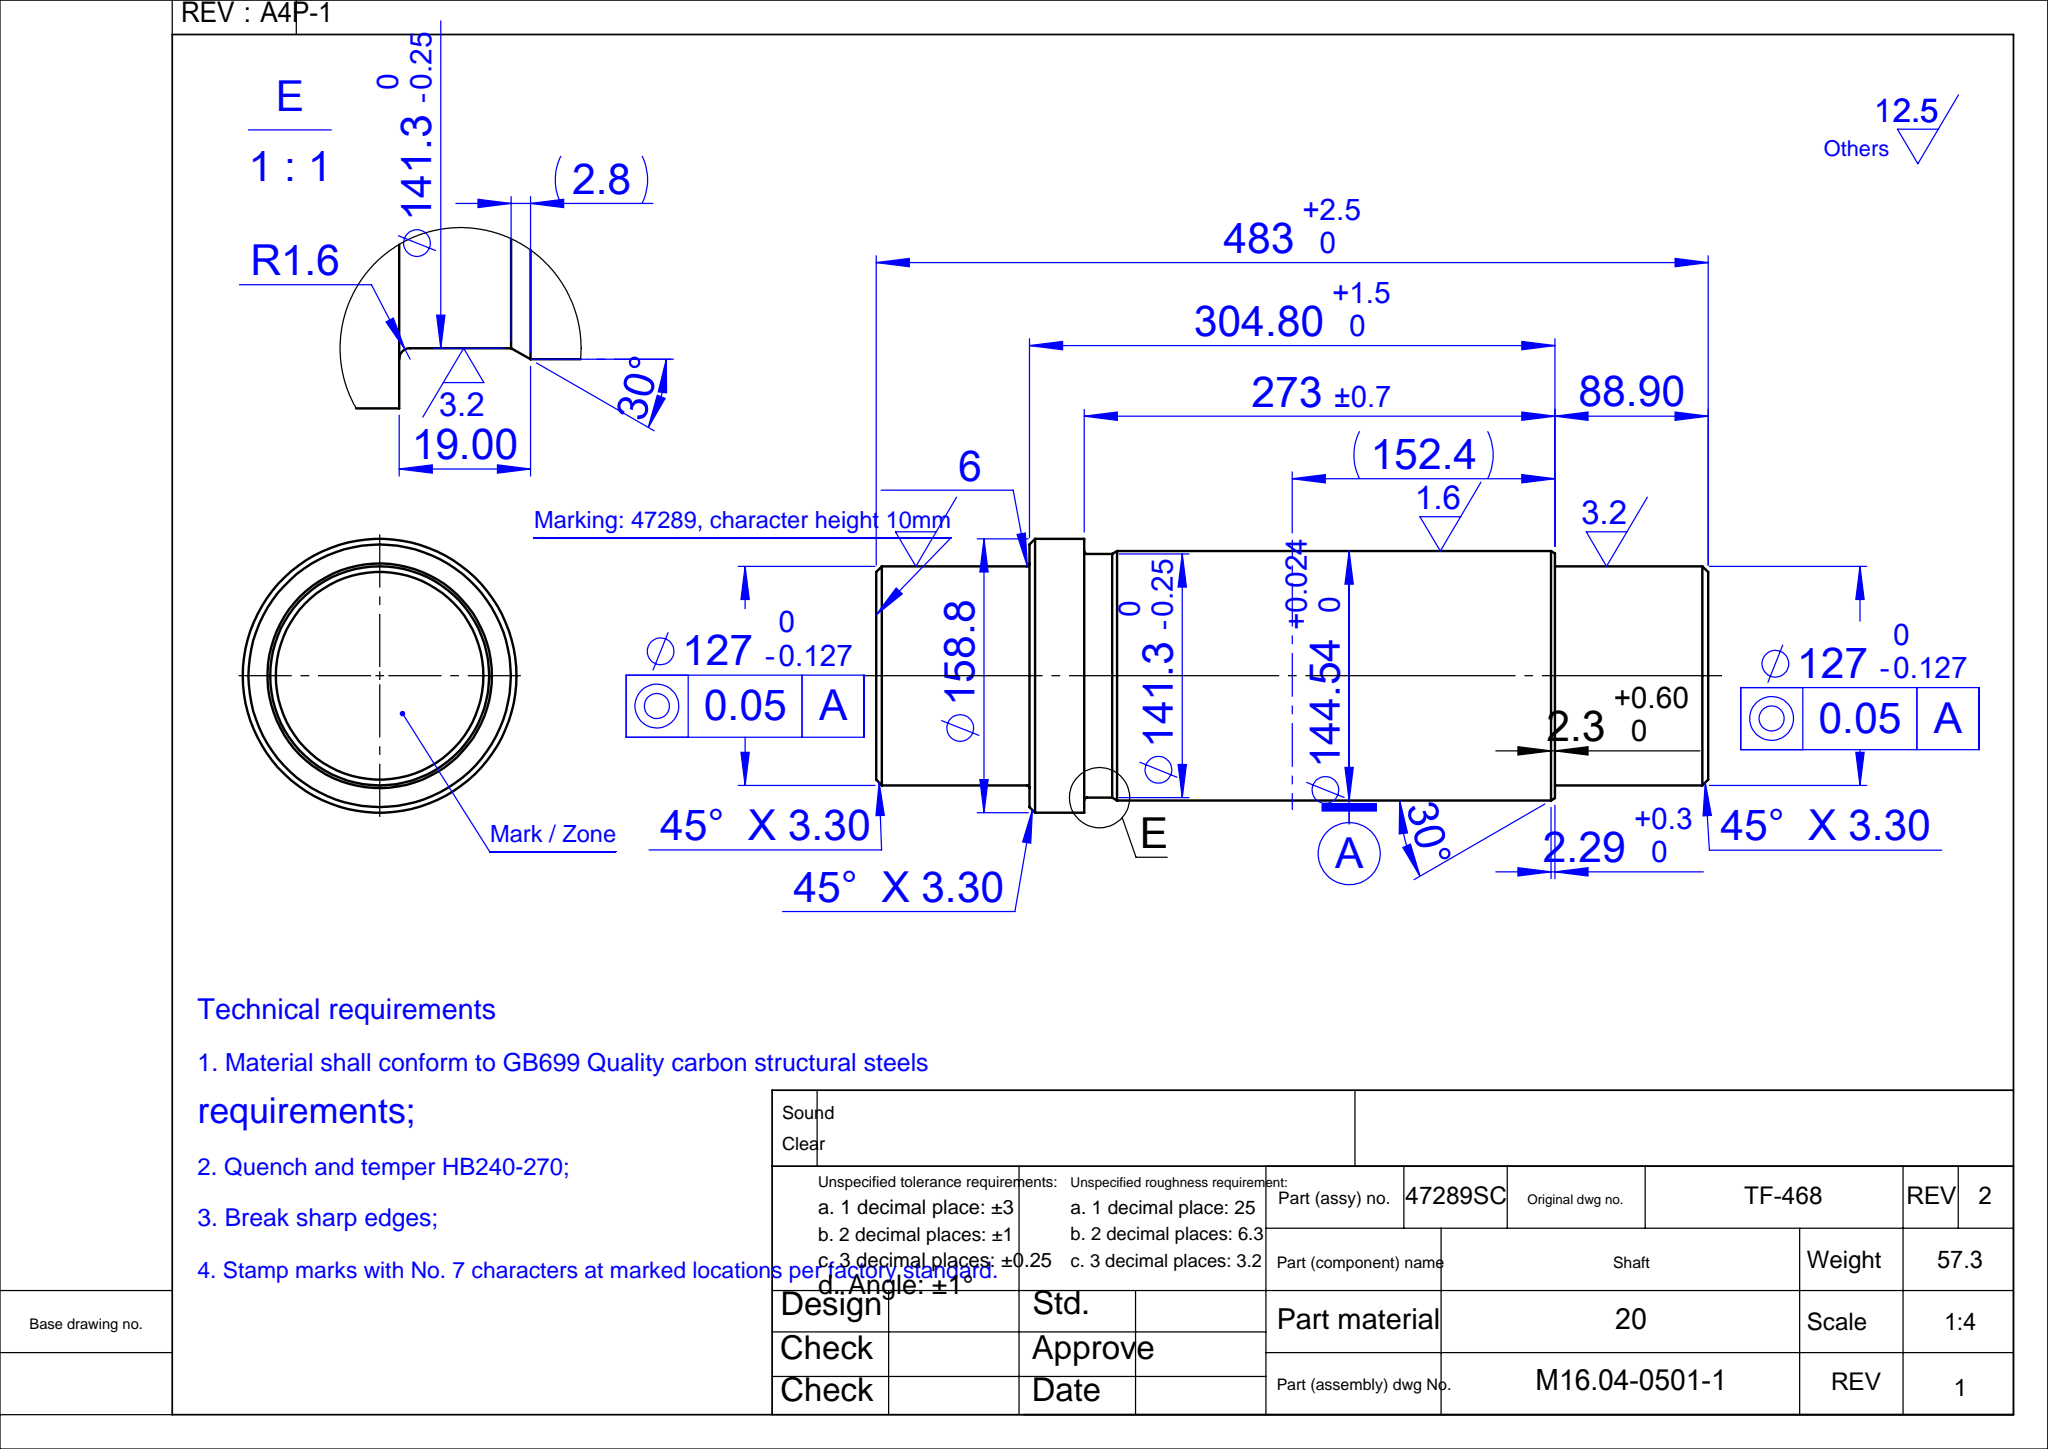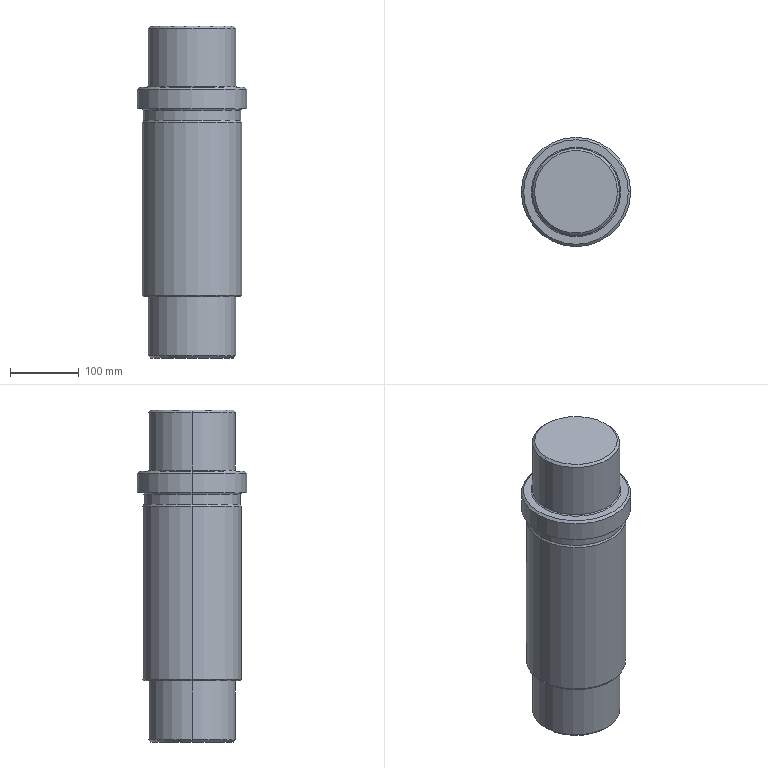Part | SolidWorks | features Revolution 1 | 1 solid | 29 faces | box 158.75 x 158.75 x 482.6 mm | volume 7340968 mm3 | cylinder 10 | cone 10 | plane 5 | torus 4 | commonest cylinder face diameters 127 x4 141.3 x2 144.539 x2 158.75 x2
STEP:
#1=CARTESIAN_POINT('',(-72.238,0.,120.65));
#2=VERTEX_POINT('',#1);
#3=CARTESIAN_POINT('',(72.238,0.,120.65));
#4=VERTEX_POINT('',#3);
#5=CARTESIAN_POINT('',(0.,0.,120.65));
#6=DIRECTION('',(0.,0.,1.));
#7=DIRECTION('',(1.,0.,0.));
#8=AXIS2_PLACEMENT_3D('',#5,#6,#7);
#9=CIRCLE('',#8,72.238);
#10=EDGE_CURVE('',#2,#4,#9,.T.);
#11=ORIENTED_EDGE('',*,*,#10,.F.);
#12=CARTESIAN_POINT('',(-70.65,0.,119.063));
#13=VERTEX_POINT('',#12);
#14=CARTESIAN_POINT('',(-72.238,0.,119.062));
#15=DIRECTION('',(0.,1.,0.));
#16=DIRECTION('',(-1.,0.,0.));
#17=AXIS2_PLACEMENT_3D('',#14,#15,#16);
#18=CIRCLE('',#17,1.588);
#19=EDGE_CURVE('',#2,#13,#18,.T.);
#20=ORIENTED_EDGE('',*,*,#19,.T.);
#21=CARTESIAN_POINT('',(70.65,0.,119.063));
#22=VERTEX_POINT('',#21);
#23=CARTESIAN_POINT('',(0.,0.,119.063));
#24=DIRECTION('',(0.,0.,1.));
#25=DIRECTION('',(1.,0.,0.));
#26=AXIS2_PLACEMENT_3D('',#23,#24,#25);
#27=CIRCLE('',#26,70.65);
#28=EDGE_CURVE('',#13,#22,#27,.T.);
#29=ORIENTED_EDGE('',*,*,#28,.T.);
#30=CARTESIAN_POINT('',(72.238,0.,119.062));
#31=DIRECTION('',(0.,-1.,0.));
#32=DIRECTION('',(0.,0.,-1.));
#33=AXIS2_PLACEMENT_3D('',#30,#31,#32);
#34=CIRCLE('',#33,1.588);
#35=EDGE_CURVE('',#4,#22,#34,.T.);
#36=ORIENTED_EDGE('',*,*,#35,.F.);
#37=EDGE_LOOP('',(#11,#20,#29,#36));
#38=FACE_OUTER_BOUND('',#37,.T.);
#39=CARTESIAN_POINT('',(0.,0.,119.062));
#40=DIRECTION('',(0.,0.,1.));
#41=DIRECTION('',(1.,0.,0.));
#42=AXIS2_PLACEMENT_3D('',#39,#40,#41);
#43=TOROIDAL_SURFACE('',#42,72.238,1.588);
#44=ADVANCED_FACE('',(#38),#43,.F.);
#45=CARTESIAN_POINT('',(70.65,0.,104.405));
#46=VERTEX_POINT('',#45);
#47=CARTESIAN_POINT('',(-70.65,0.,104.405));
#48=VERTEX_POINT('',#47);
#49=CARTESIAN_POINT('',(0.,0.,104.405));
#50=DIRECTION('',(0.,0.,1.));
#51=DIRECTION('',(1.,0.,0.));
#52=AXIS2_PLACEMENT_3D('',#49,#50,#51);
#53=CIRCLE('',#52,70.65);
#54=EDGE_CURVE('',#46,#48,#53,.T.);
#55=ORIENTED_EDGE('',*,*,#54,.T.);
#56=CARTESIAN_POINT('',(-70.65,0.,264.579));
#57=DIRECTION('',(0.,0.,1.));
#58=VECTOR('',#57,1000.);
#59=LINE('',#56,#58);
#60=EDGE_CURVE('',#48,#13,#59,.T.);
#61=ORIENTED_EDGE('',*,*,#60,.T.);
#62=CARTESIAN_POINT('',(0.,0.,119.063));
#63=DIRECTION('',(0.,0.,1.));
#64=DIRECTION('',(1.,0.,0.));
#65=AXIS2_PLACEMENT_3D('',#62,#63,#64);
#66=CIRCLE('',#65,70.65);
#67=EDGE_CURVE('',#22,#13,#66,.T.);
#68=ORIENTED_EDGE('',*,*,#67,.F.);
#69=CARTESIAN_POINT('',(70.65,0.,264.579));
#70=DIRECTION('',(0.,0.,1.));
#71=VECTOR('',#70,1000.);
#72=LINE('',#69,#71);
#73=EDGE_CURVE('',#46,#22,#72,.T.);
#74=ORIENTED_EDGE('',*,*,#73,.F.);
#75=EDGE_LOOP('',(#55,#61,#68,#74));
#76=FACE_OUTER_BOUND('',#75,.T.);
#77=CARTESIAN_POINT('',(0.,0.,264.579));
#78=DIRECTION('',(0.,0.,1.));
#79=DIRECTION('',(1.,0.,0.));
#80=AXIS2_PLACEMENT_3D('',#77,#78,#79);
#81=CYLINDRICAL_SURFACE('',#80,70.65);
#82=ADVANCED_FACE('',(#76),#81,.T.);
#83=ORIENTED_EDGE('',*,*,#54,.F.);
#84=CARTESIAN_POINT('',(72.269,0.,101.6));
#85=VERTEX_POINT('',#84);
#86=CARTESIAN_POINT('',(72.269,0.,101.6));
#87=DIRECTION('',(0.5,0.,-0.866));
#88=VECTOR('',#87,1000.);
#89=LINE('',#86,#88);
#90=EDGE_CURVE('',#46,#85,#89,.T.);
#91=ORIENTED_EDGE('',*,*,#90,.T.);
#92=CARTESIAN_POINT('',(-72.269,0.,101.6));
#93=VERTEX_POINT('',#92);
#94=CARTESIAN_POINT('',(0.,0.,101.6));
#95=DIRECTION('',(0.,0.,1.));
#96=DIRECTION('',(1.,0.,0.));
#97=AXIS2_PLACEMENT_3D('',#94,#95,#96);
#98=CIRCLE('',#97,72.269);
#99=EDGE_CURVE('',#85,#93,#98,.T.);
#100=ORIENTED_EDGE('',*,*,#99,.T.);
#101=CARTESIAN_POINT('',(-72.269,0.,101.6));
#102=DIRECTION('',(-0.5,0.,-0.866));
#103=VECTOR('',#102,1000.);
#104=LINE('',#101,#103);
#105=EDGE_CURVE('',#48,#93,#104,.T.);
#106=ORIENTED_EDGE('',*,*,#105,.F.);
#107=EDGE_LOOP('',(#83,#91,#100,#106));
#108=FACE_OUTER_BOUND('',#107,.T.);
#109=CARTESIAN_POINT('',(0.,0.,101.6));
#110=DIRECTION('',(0.,0.,-1.));
#111=DIRECTION('',(-1.,0.,0.));
#112=AXIS2_PLACEMENT_3D('',#109,#110,#111);
#113=CONICAL_SURFACE('',#112,72.269,0.5236);
#114=ADVANCED_FACE('',(#108),#113,.T.);
#115=CARTESIAN_POINT('',(72.269,0.,-150.114));
#116=VERTEX_POINT('',#115);
#117=CARTESIAN_POINT('',(-72.269,0.,-150.114));
#118=VERTEX_POINT('',#117);
#119=CARTESIAN_POINT('',(0.,0.,-150.114));
#120=DIRECTION('',(0.,0.,1.));
#121=DIRECTION('',(1.,0.,0.));
#122=AXIS2_PLACEMENT_3D('',#119,#120,#121);
#123=CIRCLE('',#122,72.269);
#124=EDGE_CURVE('',#116,#118,#123,.T.);
#125=ORIENTED_EDGE('',*,*,#124,.T.);
#126=CARTESIAN_POINT('',(-72.269,0.,264.579));
#127=DIRECTION('',(0.,0.,1.));
#128=VECTOR('',#127,1000.);
#129=LINE('',#126,#128);
#130=EDGE_CURVE('',#118,#93,#129,.T.);
#131=ORIENTED_EDGE('',*,*,#130,.T.);
#132=ORIENTED_EDGE('',*,*,#99,.F.);
#133=CARTESIAN_POINT('',(72.269,0.,264.579));
#134=DIRECTION('',(0.,0.,1.));
#135=VECTOR('',#134,1000.);
#136=LINE('',#133,#135);
#137=EDGE_CURVE('',#116,#85,#136,.T.);
#138=ORIENTED_EDGE('',*,*,#137,.F.);
#139=EDGE_LOOP('',(#125,#131,#132,#138));
#140=FACE_OUTER_BOUND('',#139,.T.);
#141=CARTESIAN_POINT('',(0.,0.,264.579));
#142=DIRECTION('',(0.,0.,1.));
#143=DIRECTION('',(1.,0.,0.));
#144=AXIS2_PLACEMENT_3D('',#141,#142,#143);
#145=CYLINDRICAL_SURFACE('',#144,72.269);
#146=ADVANCED_FACE('',(#140),#145,.T.);
#147=CARTESIAN_POINT('',(70.95,0.,-152.4));
#148=VERTEX_POINT('',#147);
#149=CARTESIAN_POINT('',(-70.95,0.,-152.4));
#150=VERTEX_POINT('',#149);
#151=CARTESIAN_POINT('',(0.,0.,-152.4));
#152=DIRECTION('',(0.,0.,1.));
#153=DIRECTION('',(1.,0.,0.));
#154=AXIS2_PLACEMENT_3D('',#151,#152,#153);
#155=CIRCLE('',#154,70.95);
#156=EDGE_CURVE('',#148,#150,#155,.T.);
#157=ORIENTED_EDGE('',*,*,#156,.T.);
#158=CARTESIAN_POINT('',(-70.95,0.,-152.4));
#159=DIRECTION('',(-0.5,0.,0.866));
#160=VECTOR('',#159,1000.);
#161=LINE('',#158,#160);
#162=EDGE_CURVE('',#150,#118,#161,.T.);
#163=ORIENTED_EDGE('',*,*,#162,.T.);
#164=ORIENTED_EDGE('',*,*,#124,.F.);
#165=CARTESIAN_POINT('',(70.95,0.,-152.4));
#166=DIRECTION('',(0.5,0.,0.866));
#167=VECTOR('',#166,1000.);
#168=LINE('',#165,#167);
#169=EDGE_CURVE('',#148,#116,#168,.T.);
#170=ORIENTED_EDGE('',*,*,#169,.F.);
#171=EDGE_LOOP('',(#157,#163,#164,#170));
#172=FACE_OUTER_BOUND('',#171,.T.);
#173=CARTESIAN_POINT('',(0.,0.,-152.4));
#174=DIRECTION('',(0.,0.,1.));
#175=DIRECTION('',(1.,0.,0.));
#176=AXIS2_PLACEMENT_3D('',#173,#174,#175);
#177=CONICAL_SURFACE('',#176,70.95,0.5236);
#178=ADVANCED_FACE('',(#172),#177,.T.);
#179=CARTESIAN_POINT('',(63.5,0.,-237.998));
#180=VERTEX_POINT('',#179);
#181=CARTESIAN_POINT('',(-63.5,0.,-237.998));
#182=VERTEX_POINT('',#181);
#183=CARTESIAN_POINT('',(0.,0.,-237.998));
#184=DIRECTION('',(0.,0.,1.));
#185=DIRECTION('',(1.,0.,0.));
#186=AXIS2_PLACEMENT_3D('',#183,#184,#185);
#187=CIRCLE('',#186,63.5);
#188=EDGE_CURVE('',#180,#182,#187,.T.);
#189=ORIENTED_EDGE('',*,*,#188,.T.);
#190=CARTESIAN_POINT('',(-63.5,0.,-152.4));
#191=VERTEX_POINT('',#190);
#192=CARTESIAN_POINT('',(-63.5,0.,264.579));
#193=DIRECTION('',(0.,0.,1.));
#194=VECTOR('',#193,1000.);
#195=LINE('',#192,#194);
#196=EDGE_CURVE('',#182,#191,#195,.T.);
#197=ORIENTED_EDGE('',*,*,#196,.T.);
#198=CARTESIAN_POINT('',(63.5,0.,-152.4));
#199=VERTEX_POINT('',#198);
#200=CARTESIAN_POINT('',(0.,0.,-152.4));
#201=DIRECTION('',(0.,0.,1.));
#202=DIRECTION('',(1.,0.,0.));
#203=AXIS2_PLACEMENT_3D('',#200,#201,#202);
#204=CIRCLE('',#203,63.5);
#205=EDGE_CURVE('',#199,#191,#204,.T.);
#206=ORIENTED_EDGE('',*,*,#205,.F.);
#207=CARTESIAN_POINT('',(63.5,0.,264.579));
#208=DIRECTION('',(0.,0.,1.));
#209=VECTOR('',#208,1000.);
#210=LINE('',#207,#209);
#211=EDGE_CURVE('',#180,#199,#210,.T.);
#212=ORIENTED_EDGE('',*,*,#211,.F.);
#213=EDGE_LOOP('',(#189,#197,#206,#212));
#214=FACE_OUTER_BOUND('',#213,.T.);
#215=CARTESIAN_POINT('',(0.,0.,264.579));
#216=DIRECTION('',(0.,0.,1.));
#217=DIRECTION('',(1.,0.,0.));
#218=AXIS2_PLACEMENT_3D('',#215,#216,#217);
#219=CYLINDRICAL_SURFACE('',#218,63.5);
#220=ADVANCED_FACE('',(#214),#219,.T.);
#221=CARTESIAN_POINT('',(60.198,0.,-241.3));
#222=VERTEX_POINT('',#221);
#223=CARTESIAN_POINT('',(-60.198,0.,-241.3));
#224=VERTEX_POINT('',#223);
#225=CARTESIAN_POINT('',(0.,0.,-241.3));
#226=DIRECTION('',(0.,0.,1.));
#227=DIRECTION('',(1.,0.,0.));
#228=AXIS2_PLACEMENT_3D('',#225,#226,#227);
#229=CIRCLE('',#228,60.198);
#230=EDGE_CURVE('',#222,#224,#229,.T.);
#231=ORIENTED_EDGE('',*,*,#230,.T.);
#232=CARTESIAN_POINT('',(-60.198,0.,-241.3));
#233=DIRECTION('',(-0.7071,0.,0.7071));
#234=VECTOR('',#233,1000.);
#235=LINE('',#232,#234);
#236=EDGE_CURVE('',#224,#182,#235,.T.);
#237=ORIENTED_EDGE('',*,*,#236,.T.);
#238=ORIENTED_EDGE('',*,*,#188,.F.);
#239=CARTESIAN_POINT('',(60.198,0.,-241.3));
#240=DIRECTION('',(0.7071,0.,0.7071));
#241=VECTOR('',#240,1000.);
#242=LINE('',#239,#241);
#243=EDGE_CURVE('',#222,#180,#242,.T.);
#244=ORIENTED_EDGE('',*,*,#243,.F.);
#245=EDGE_LOOP('',(#231,#237,#238,#244));
#246=FACE_OUTER_BOUND('',#245,.T.);
#247=CARTESIAN_POINT('',(0.,0.,-241.3));
#248=DIRECTION('',(0.,0.,1.));
#249=DIRECTION('',(1.,0.,0.));
#250=AXIS2_PLACEMENT_3D('',#247,#248,#249);
#251=CONICAL_SURFACE('',#250,60.198,0.7854);
#252=ADVANCED_FACE('',(#246),#251,.T.);
#253=CARTESIAN_POINT('',(60.198,0.,241.3));
#254=VERTEX_POINT('',#253);
#255=CARTESIAN_POINT('',(-60.198,0.,241.3));
#256=VERTEX_POINT('',#255);
#257=CARTESIAN_POINT('',(0.,0.,241.3));
#258=DIRECTION('',(0.,0.,1.));
#259=DIRECTION('',(1.,0.,0.));
#260=AXIS2_PLACEMENT_3D('',#257,#258,#259);
#261=CIRCLE('',#260,60.198);
#262=EDGE_CURVE('',#254,#256,#261,.T.);
#263=ORIENTED_EDGE('',*,*,#262,.F.);
#264=CARTESIAN_POINT('',(63.5,0.,237.998));
#265=VERTEX_POINT('',#264);
#266=CARTESIAN_POINT('',(63.5,0.,237.998));
#267=DIRECTION('',(0.7071,0.,-0.7071));
#268=VECTOR('',#267,1000.);
#269=LINE('',#266,#268);
#270=EDGE_CURVE('',#254,#265,#269,.T.);
#271=ORIENTED_EDGE('',*,*,#270,.T.);
#272=CARTESIAN_POINT('',(-63.5,0.,237.998));
#273=VERTEX_POINT('',#272);
#274=CARTESIAN_POINT('',(0.,0.,237.998));
#275=DIRECTION('',(0.,0.,1.));
#276=DIRECTION('',(1.,0.,0.));
#277=AXIS2_PLACEMENT_3D('',#274,#275,#276);
#278=CIRCLE('',#277,63.5);
#279=EDGE_CURVE('',#265,#273,#278,.T.);
#280=ORIENTED_EDGE('',*,*,#279,.T.);
#281=CARTESIAN_POINT('',(-63.5,0.,237.998));
#282=DIRECTION('',(-0.7071,0.,-0.7071));
#283=VECTOR('',#282,1000.);
#284=LINE('',#281,#283);
#285=EDGE_CURVE('',#256,#273,#284,.T.);
#286=ORIENTED_EDGE('',*,*,#285,.F.);
#287=EDGE_LOOP('',(#263,#271,#280,#286));
#288=FACE_OUTER_BOUND('',#287,.T.);
#289=CARTESIAN_POINT('',(0.,0.,237.998));
#290=DIRECTION('',(0.,0.,-1.));
#291=DIRECTION('',(-1.,0.,0.));
#292=AXIS2_PLACEMENT_3D('',#289,#290,#291);
#293=CONICAL_SURFACE('',#292,63.5,0.7854);
#294=ADVANCED_FACE('',(#288),#293,.T.);
#295=CARTESIAN_POINT('',(63.5,0.,153.988));
#296=VERTEX_POINT('',#295);
#297=CARTESIAN_POINT('',(-63.5,0.,153.988));
#298=VERTEX_POINT('',#297);
#299=CARTESIAN_POINT('',(0.,0.,153.988));
#300=DIRECTION('',(0.,0.,1.));
#301=DIRECTION('',(1.,0.,0.));
#302=AXIS2_PLACEMENT_3D('',#299,#300,#301);
#303=CIRCLE('',#302,63.5);
#304=EDGE_CURVE('',#296,#298,#303,.T.);
#305=ORIENTED_EDGE('',*,*,#304,.T.);
#306=CARTESIAN_POINT('',(-63.5,0.,264.579));
#307=DIRECTION('',(0.,0.,1.));
#308=VECTOR('',#307,1000.);
#309=LINE('',#306,#308);
#310=EDGE_CURVE('',#298,#273,#309,.T.);
#311=ORIENTED_EDGE('',*,*,#310,.T.);
#312=ORIENTED_EDGE('',*,*,#279,.F.);
#313=CARTESIAN_POINT('',(63.5,0.,264.579));
#314=DIRECTION('',(0.,0.,1.));
#315=VECTOR('',#314,1000.);
#316=LINE('',#313,#315);
#317=EDGE_CURVE('',#296,#265,#316,.T.);
#318=ORIENTED_EDGE('',*,*,#317,.F.);
#319=EDGE_LOOP('',(#305,#311,#312,#318));
#320=FACE_OUTER_BOUND('',#319,.T.);
#321=CARTESIAN_POINT('',(0.,0.,264.579));
#322=DIRECTION('',(0.,0.,1.));
#323=DIRECTION('',(1.,0.,0.));
#324=AXIS2_PLACEMENT_3D('',#321,#322,#323);
#325=CYLINDRICAL_SURFACE('',#324,63.5);
#326=ADVANCED_FACE('',(#320),#325,.T.);
#327=CARTESIAN_POINT('',(0.,0.,153.988));
#328=DIRECTION('',(0.,0.,1.));
#329=DIRECTION('',(1.,0.,0.));
#330=AXIS2_PLACEMENT_3D('',#327,#328,#329);
#331=CIRCLE('',#330,63.5);
#332=EDGE_CURVE('',#298,#296,#331,.T.);
#333=ORIENTED_EDGE('',*,*,#332,.F.);
#334=CARTESIAN_POINT('',(-65.088,0.,152.4));
#335=VERTEX_POINT('',#334);
#336=CARTESIAN_POINT('',(-65.088,0.,153.988));
#337=DIRECTION('',(0.,1.,0.));
#338=DIRECTION('',(-1.,0.,0.));
#339=AXIS2_PLACEMENT_3D('',#336,#337,#338);
#340=CIRCLE('',#339,1.588);
#341=EDGE_CURVE('',#298,#335,#340,.T.);
#342=ORIENTED_EDGE('',*,*,#341,.T.);
#343=CARTESIAN_POINT('',(65.088,0.,152.4));
#344=VERTEX_POINT('',#343);
#345=CARTESIAN_POINT('',(0.,0.,152.4));
#346=DIRECTION('',(0.,0.,1.));
#347=DIRECTION('',(1.,0.,0.));
#348=AXIS2_PLACEMENT_3D('',#345,#346,#347);
#349=CIRCLE('',#348,65.088);
#350=EDGE_CURVE('',#335,#344,#349,.T.);
#351=ORIENTED_EDGE('',*,*,#350,.T.);
#352=CARTESIAN_POINT('',(65.088,0.,153.988));
#353=DIRECTION('',(0.,-1.,0.));
#354=DIRECTION('',(0.,0.,-1.));
#355=AXIS2_PLACEMENT_3D('',#352,#353,#354);
#356=CIRCLE('',#355,1.587);
#357=EDGE_CURVE('',#296,#344,#356,.T.);
#358=ORIENTED_EDGE('',*,*,#357,.F.);
#359=EDGE_LOOP('',(#333,#342,#351,#358));
#360=FACE_OUTER_BOUND('',#359,.T.);
#361=CARTESIAN_POINT('',(0.,0.,153.988));
#362=DIRECTION('',(0.,0.,1.));
#363=DIRECTION('',(1.,0.,0.));
#364=AXIS2_PLACEMENT_3D('',#361,#362,#363);
#365=TOROIDAL_SURFACE('',#364,65.088,1.587);
#366=ADVANCED_FACE('',(#360),#365,.F.);
#367=CARTESIAN_POINT('',(76.073,0.,152.4));
#368=VERTEX_POINT('',#367);
#369=CARTESIAN_POINT('',(-76.073,0.,152.4));
#370=VERTEX_POINT('',#369);
#371=CARTESIAN_POINT('',(0.,0.,152.4));
#372=DIRECTION('',(0.,0.,1.));
#373=DIRECTION('',(1.,0.,0.));
#374=AXIS2_PLACEMENT_3D('',#371,#372,#373);
#375=CIRCLE('',#374,76.073);
#376=EDGE_CURVE('',#368,#370,#375,.T.);
#377=ORIENTED_EDGE('',*,*,#376,.F.);
#378=CARTESIAN_POINT('',(79.375,0.,149.098));
#379=VERTEX_POINT('',#378);
#380=CARTESIAN_POINT('',(79.375,0.,149.098));
#381=DIRECTION('',(0.7071,0.,-0.7071));
#382=VECTOR('',#381,1000.);
#383=LINE('',#380,#382);
#384=EDGE_CURVE('',#368,#379,#383,.T.);
#385=ORIENTED_EDGE('',*,*,#384,.T.);
#386=CARTESIAN_POINT('',(-79.375,0.,149.098));
#387=VERTEX_POINT('',#386);
#388=CARTESIAN_POINT('',(0.,0.,149.098));
#389=DIRECTION('',(0.,0.,1.));
#390=DIRECTION('',(1.,0.,0.));
#391=AXIS2_PLACEMENT_3D('',#388,#389,#390);
#392=CIRCLE('',#391,79.375);
#393=EDGE_CURVE('',#379,#387,#392,.T.);
#394=ORIENTED_EDGE('',*,*,#393,.T.);
#395=CARTESIAN_POINT('',(-79.375,0.,149.098));
#396=DIRECTION('',(-0.7071,0.,-0.7071));
#397=VECTOR('',#396,1000.);
#398=LINE('',#395,#397);
#399=EDGE_CURVE('',#370,#387,#398,.T.);
#400=ORIENTED_EDGE('',*,*,#399,.F.);
#401=EDGE_LOOP('',(#377,#385,#394,#400));
#402=FACE_OUTER_BOUND('',#401,.T.);
#403=CARTESIAN_POINT('',(0.,0.,149.098));
#404=DIRECTION('',(0.,0.,-1.));
#405=DIRECTION('',(-1.,0.,0.));
#406=AXIS2_PLACEMENT_3D('',#403,#404,#405);
#407=CONICAL_SURFACE('',#406,79.375,0.7854);
#408=ADVANCED_FACE('',(#402),#407,.T.);
#409=CARTESIAN_POINT('',(79.375,0.,120.65));
#410=VERTEX_POINT('',#409);
#411=CARTESIAN_POINT('',(-79.375,0.,120.65));
#412=VERTEX_POINT('',#411);
#413=CARTESIAN_POINT('',(0.,0.,120.65));
#414=DIRECTION('',(0.,0.,1.));
#415=DIRECTION('',(1.,0.,0.));
#416=AXIS2_PLACEMENT_3D('',#413,#414,#415);
#417=CIRCLE('',#416,79.375);
#418=EDGE_CURVE('',#410,#412,#417,.T.);
#419=ORIENTED_EDGE('',*,*,#418,.T.);
#420=CARTESIAN_POINT('',(-79.375,0.,264.579));
#421=DIRECTION('',(0.,0.,1.));
#422=VECTOR('',#421,1000.);
#423=LINE('',#420,#422);
#424=EDGE_CURVE('',#412,#387,#423,.T.);
#425=ORIENTED_EDGE('',*,*,#424,.T.);
#426=ORIENTED_EDGE('',*,*,#393,.F.);
#427=CARTESIAN_POINT('',(79.375,0.,264.579));
#428=DIRECTION('',(0.,0.,1.));
#429=VECTOR('',#428,1000.);
#430=LINE('',#427,#429);
#431=EDGE_CURVE('',#410,#379,#430,.T.);
#432=ORIENTED_EDGE('',*,*,#431,.F.);
#433=EDGE_LOOP('',(#419,#425,#426,#432));
#434=FACE_OUTER_BOUND('',#433,.T.);
#435=CARTESIAN_POINT('',(0.,0.,264.579));
#436=DIRECTION('',(0.,0.,1.));
#437=DIRECTION('',(1.,0.,0.));
#438=AXIS2_PLACEMENT_3D('',#435,#436,#437);
#439=CYLINDRICAL_SURFACE('',#438,79.375);
#440=ADVANCED_FACE('',(#434),#439,.T.);
#441=ORIENTED_EDGE('',*,*,#418,.F.);
#442=CARTESIAN_POINT('',(0.,0.,120.65));
#443=DIRECTION('',(0.,0.,1.));
#444=DIRECTION('',(1.,0.,0.));
#445=AXIS2_PLACEMENT_3D('',#442,#443,#444);
#446=CIRCLE('',#445,79.375);
#447=EDGE_CURVE('',#412,#410,#446,.T.);
#448=ORIENTED_EDGE('',*,*,#447,.F.);
#449=EDGE_LOOP('',(#441,#448));
#450=FACE_OUTER_BOUND('',#449,.T.);
#451=CARTESIAN_POINT('',(0.,0.,120.65));
#452=DIRECTION('',(0.,0.,1.));
#453=DIRECTION('',(1.,0.,0.));
#454=AXIS2_PLACEMENT_3D('',#451,#452,#453);
#455=CIRCLE('',#454,72.238);
#456=EDGE_CURVE('',#4,#2,#455,.T.);
#457=ORIENTED_EDGE('',*,*,#456,.T.);
#458=ORIENTED_EDGE('',*,*,#10,.T.);
#459=EDGE_LOOP('',(#457,#458));
#460=FACE_BOUND('',#459,.T.);
#461=CARTESIAN_POINT('',(0.,79.375,120.65));
#462=DIRECTION('',(0.,0.,1.));
#463=DIRECTION('',(1.,0.,0.));
#464=AXIS2_PLACEMENT_3D('',#461,#462,#463);
#465=PLANE('',#464);
#466=ADVANCED_FACE('',(#450,#460),#465,.F.);
#467=ORIENTED_EDGE('',*,*,#424,.F.);
#468=ORIENTED_EDGE('',*,*,#447,.T.);
#469=ORIENTED_EDGE('',*,*,#431,.T.);
#470=CARTESIAN_POINT('',(0.,0.,149.098));
#471=DIRECTION('',(0.,0.,1.));
#472=DIRECTION('',(1.,0.,0.));
#473=AXIS2_PLACEMENT_3D('',#470,#471,#472);
#474=CIRCLE('',#473,79.375);
#475=EDGE_CURVE('',#387,#379,#474,.T.);
#476=ORIENTED_EDGE('',*,*,#475,.F.);
#477=EDGE_LOOP('',(#467,#468,#469,#476));
#478=FACE_OUTER_BOUND('',#477,.T.);
#479=CARTESIAN_POINT('',(0.,0.,264.579));
#480=DIRECTION('',(0.,0.,1.));
#481=DIRECTION('',(1.,0.,0.));
#482=AXIS2_PLACEMENT_3D('',#479,#480,#481);
#483=CYLINDRICAL_SURFACE('',#482,79.375);
#484=ADVANCED_FACE('',(#478),#483,.T.);
#485=ORIENTED_EDGE('',*,*,#384,.F.);
#486=CARTESIAN_POINT('',(0.,0.,152.4));
#487=DIRECTION('',(0.,0.,1.));
#488=DIRECTION('',(1.,0.,0.));
#489=AXIS2_PLACEMENT_3D('',#486,#487,#488);
#490=CIRCLE('',#489,76.073);
#491=EDGE_CURVE('',#370,#368,#490,.T.);
#492=ORIENTED_EDGE('',*,*,#491,.F.);
#493=ORIENTED_EDGE('',*,*,#399,.T.);
#494=ORIENTED_EDGE('',*,*,#475,.T.);
#495=EDGE_LOOP('',(#485,#492,#493,#494));
#496=FACE_OUTER_BOUND('',#495,.T.);
#497=CARTESIAN_POINT('',(0.,0.,149.098));
#498=DIRECTION('',(0.,0.,-1.));
#499=DIRECTION('',(-1.,0.,0.));
#500=AXIS2_PLACEMENT_3D('',#497,#498,#499);
#501=CONICAL_SURFACE('',#500,79.375,0.7854);
#502=ADVANCED_FACE('',(#496),#501,.T.);
#503=CARTESIAN_POINT('',(0.,0.,152.4));
#504=DIRECTION('',(0.,0.,1.));
#505=DIRECTION('',(1.,0.,0.));
#506=AXIS2_PLACEMENT_3D('',#503,#504,#505);
#507=CIRCLE('',#506,65.088);
#508=EDGE_CURVE('',#344,#335,#507,.T.);
#509=ORIENTED_EDGE('',*,*,#508,.F.);
#510=ORIENTED_EDGE('',*,*,#350,.F.);
#511=EDGE_LOOP('',(#509,#510));
#512=FACE_BOUND('',#511,.T.);
#513=ORIENTED_EDGE('',*,*,#491,.T.);
#514=ORIENTED_EDGE('',*,*,#376,.T.);
#515=EDGE_LOOP('',(#513,#514));
#516=FACE_OUTER_BOUND('',#515,.T.);
#517=CARTESIAN_POINT('',(0.,65.088,152.4));
#518=DIRECTION('',(0.,0.,-1.));
#519=DIRECTION('',(-1.,0.,0.));
#520=AXIS2_PLACEMENT_3D('',#517,#518,#519);
#521=PLANE('',#520);
#522=ADVANCED_FACE('',(#512,#516),#521,.F.);
#523=ORIENTED_EDGE('',*,*,#341,.F.);
#524=ORIENTED_EDGE('',*,*,#304,.F.);
#525=ORIENTED_EDGE('',*,*,#357,.T.);
#526=ORIENTED_EDGE('',*,*,#508,.T.);
#527=EDGE_LOOP('',(#523,#524,#525,#526));
#528=FACE_OUTER_BOUND('',#527,.T.);
#529=CARTESIAN_POINT('',(0.,0.,153.988));
#530=DIRECTION('',(0.,0.,1.));
#531=DIRECTION('',(1.,0.,0.));
#532=AXIS2_PLACEMENT_3D('',#529,#530,#531);
#533=TOROIDAL_SURFACE('',#532,65.088,1.587);
#534=ADVANCED_FACE('',(#528),#533,.F.);
#535=ORIENTED_EDGE('',*,*,#310,.F.);
#536=ORIENTED_EDGE('',*,*,#332,.T.);
#537=ORIENTED_EDGE('',*,*,#317,.T.);
#538=CARTESIAN_POINT('',(0.,0.,237.998));
#539=DIRECTION('',(0.,0.,1.));
#540=DIRECTION('',(1.,0.,0.));
#541=AXIS2_PLACEMENT_3D('',#538,#539,#540);
#542=CIRCLE('',#541,63.5);
#543=EDGE_CURVE('',#273,#265,#542,.T.);
#544=ORIENTED_EDGE('',*,*,#543,.F.);
#545=EDGE_LOOP('',(#535,#536,#537,#544));
#546=FACE_OUTER_BOUND('',#545,.T.);
#547=CARTESIAN_POINT('',(0.,0.,264.579));
#548=DIRECTION('',(0.,0.,1.));
#549=DIRECTION('',(1.,0.,0.));
#550=AXIS2_PLACEMENT_3D('',#547,#548,#549);
#551=CYLINDRICAL_SURFACE('',#550,63.5);
#552=ADVANCED_FACE('',(#546),#551,.T.);
#553=ORIENTED_EDGE('',*,*,#270,.F.);
#554=CARTESIAN_POINT('',(0.,0.,241.3));
#555=DIRECTION('',(0.,0.,1.));
#556=DIRECTION('',(1.,0.,0.));
#557=AXIS2_PLACEMENT_3D('',#554,#555,#556);
#558=CIRCLE('',#557,60.198);
#559=EDGE_CURVE('',#256,#254,#558,.T.);
#560=ORIENTED_EDGE('',*,*,#559,.F.);
#561=ORIENTED_EDGE('',*,*,#285,.T.);
#562=ORIENTED_EDGE('',*,*,#543,.T.);
#563=EDGE_LOOP('',(#553,#560,#561,#562));
#564=FACE_OUTER_BOUND('',#563,.T.);
#565=CARTESIAN_POINT('',(0.,0.,237.998));
#566=DIRECTION('',(0.,0.,-1.));
#567=DIRECTION('',(-1.,0.,0.));
#568=AXIS2_PLACEMENT_3D('',#565,#566,#567);
#569=CONICAL_SURFACE('',#568,63.5,0.7854);
#570=ADVANCED_FACE('',(#564),#569,.T.);
#571=ORIENTED_EDGE('',*,*,#559,.T.);
#572=ORIENTED_EDGE('',*,*,#262,.T.);
#573=EDGE_LOOP('',(#571,#572));
#574=FACE_OUTER_BOUND('',#573,.T.);
#575=CARTESIAN_POINT('',(0.,60.198,241.3));
#576=DIRECTION('',(0.,0.,-1.));
#577=DIRECTION('',(-1.,0.,0.));
#578=AXIS2_PLACEMENT_3D('',#575,#576,#577);
#579=PLANE('',#578);
#580=ADVANCED_FACE('',(#574),#579,.F.);
#581=ORIENTED_EDGE('',*,*,#230,.F.);
#582=CARTESIAN_POINT('',(0.,0.,-241.3));
#583=DIRECTION('',(0.,0.,1.));
#584=DIRECTION('',(1.,0.,0.));
#585=AXIS2_PLACEMENT_3D('',#582,#583,#584);
#586=CIRCLE('',#585,60.198);
#587=EDGE_CURVE('',#224,#222,#586,.T.);
#588=ORIENTED_EDGE('',*,*,#587,.F.);
#589=EDGE_LOOP('',(#581,#588));
#590=FACE_OUTER_BOUND('',#589,.T.);
#591=CARTESIAN_POINT('',(0.,60.198,-241.3));
#592=DIRECTION('',(0.,0.,1.));
#593=DIRECTION('',(1.,0.,0.));
#594=AXIS2_PLACEMENT_3D('',#591,#592,#593);
#595=PLANE('',#594);
#596=ADVANCED_FACE('',(#590),#595,.F.);
#597=ORIENTED_EDGE('',*,*,#236,.F.);
#598=ORIENTED_EDGE('',*,*,#587,.T.);
#599=ORIENTED_EDGE('',*,*,#243,.T.);
#600=CARTESIAN_POINT('',(0.,0.,-237.998));
#601=DIRECTION('',(0.,0.,1.));
#602=DIRECTION('',(1.,0.,0.));
#603=AXIS2_PLACEMENT_3D('',#600,#601,#602);
#604=CIRCLE('',#603,63.5);
#605=EDGE_CURVE('',#182,#180,#604,.T.);
#606=ORIENTED_EDGE('',*,*,#605,.F.);
#607=EDGE_LOOP('',(#597,#598,#599,#606));
#608=FACE_OUTER_BOUND('',#607,.T.);
#609=CARTESIAN_POINT('',(0.,0.,-241.3));
#610=DIRECTION('',(0.,0.,1.));
#611=DIRECTION('',(1.,0.,0.));
#612=AXIS2_PLACEMENT_3D('',#609,#610,#611);
#613=CONICAL_SURFACE('',#612,60.198,0.7854);
#614=ADVANCED_FACE('',(#608),#613,.T.);
#615=ORIENTED_EDGE('',*,*,#196,.F.);
#616=ORIENTED_EDGE('',*,*,#605,.T.);
#617=ORIENTED_EDGE('',*,*,#211,.T.);
#618=CARTESIAN_POINT('',(0.,0.,-152.4));
#619=DIRECTION('',(0.,0.,1.));
#620=DIRECTION('',(1.,0.,0.));
#621=AXIS2_PLACEMENT_3D('',#618,#619,#620);
#622=CIRCLE('',#621,63.5);
#623=EDGE_CURVE('',#191,#199,#622,.T.);
#624=ORIENTED_EDGE('',*,*,#623,.F.);
#625=EDGE_LOOP('',(#615,#616,#617,#624));
#626=FACE_OUTER_BOUND('',#625,.T.);
#627=CARTESIAN_POINT('',(0.,0.,264.579));
#628=DIRECTION('',(0.,0.,1.));
#629=DIRECTION('',(1.,0.,0.));
#630=AXIS2_PLACEMENT_3D('',#627,#628,#629);
#631=CYLINDRICAL_SURFACE('',#630,63.5);
#632=ADVANCED_FACE('',(#626),#631,.T.);
#633=ORIENTED_EDGE('',*,*,#156,.F.);
#634=CARTESIAN_POINT('',(0.,0.,-152.4));
#635=DIRECTION('',(0.,0.,1.));
#636=DIRECTION('',(1.,0.,0.));
#637=AXIS2_PLACEMENT_3D('',#634,#635,#636);
#638=CIRCLE('',#637,70.95);
#639=EDGE_CURVE('',#150,#148,#638,.T.);
#640=ORIENTED_EDGE('',*,*,#639,.F.);
#641=EDGE_LOOP('',(#633,#640));
#642=FACE_OUTER_BOUND('',#641,.T.);
#643=ORIENTED_EDGE('',*,*,#205,.T.);
#644=ORIENTED_EDGE('',*,*,#623,.T.);
#645=EDGE_LOOP('',(#643,#644));
#646=FACE_BOUND('',#645,.T.);
#647=CARTESIAN_POINT('',(0.,70.95,-152.4));
#648=DIRECTION('',(0.,0.,1.));
#649=DIRECTION('',(1.,0.,0.));
#650=AXIS2_PLACEMENT_3D('',#647,#648,#649);
#651=PLANE('',#650);
#652=ADVANCED_FACE('',(#642,#646),#651,.F.);
#653=ORIENTED_EDGE('',*,*,#162,.F.);
#654=ORIENTED_EDGE('',*,*,#639,.T.);
#655=ORIENTED_EDGE('',*,*,#169,.T.);
#656=CARTESIAN_POINT('',(0.,0.,-150.114));
#657=DIRECTION('',(0.,0.,1.));
#658=DIRECTION('',(1.,0.,0.));
#659=AXIS2_PLACEMENT_3D('',#656,#657,#658);
#660=CIRCLE('',#659,72.269);
#661=EDGE_CURVE('',#118,#116,#660,.T.);
#662=ORIENTED_EDGE('',*,*,#661,.F.);
#663=EDGE_LOOP('',(#653,#654,#655,#662));
#664=FACE_OUTER_BOUND('',#663,.T.);
#665=CARTESIAN_POINT('',(0.,0.,-152.4));
#666=DIRECTION('',(0.,0.,1.));
#667=DIRECTION('',(1.,0.,0.));
#668=AXIS2_PLACEMENT_3D('',#665,#666,#667);
#669=CONICAL_SURFACE('',#668,70.95,0.5236);
#670=ADVANCED_FACE('',(#664),#669,.T.);
#671=ORIENTED_EDGE('',*,*,#130,.F.);
#672=ORIENTED_EDGE('',*,*,#661,.T.);
#673=ORIENTED_EDGE('',*,*,#137,.T.);
#674=CARTESIAN_POINT('',(0.,0.,101.6));
#675=DIRECTION('',(0.,0.,1.));
#676=DIRECTION('',(1.,0.,0.));
#677=AXIS2_PLACEMENT_3D('',#674,#675,#676);
#678=CIRCLE('',#677,72.269);
#679=EDGE_CURVE('',#93,#85,#678,.T.);
#680=ORIENTED_EDGE('',*,*,#679,.F.);
#681=EDGE_LOOP('',(#671,#672,#673,#680));
#682=FACE_OUTER_BOUND('',#681,.T.);
#683=CARTESIAN_POINT('',(0.,0.,264.579));
#684=DIRECTION('',(0.,0.,1.));
#685=DIRECTION('',(1.,0.,0.));
#686=AXIS2_PLACEMENT_3D('',#683,#684,#685);
#687=CYLINDRICAL_SURFACE('',#686,72.269);
#688=ADVANCED_FACE('',(#682),#687,.T.);
#689=ORIENTED_EDGE('',*,*,#90,.F.);
#690=CARTESIAN_POINT('',(0.,0.,104.405));
#691=DIRECTION('',(0.,0.,1.));
#692=DIRECTION('',(1.,0.,0.));
#693=AXIS2_PLACEMENT_3D('',#690,#691,#692);
#694=CIRCLE('',#693,70.65);
#695=EDGE_CURVE('',#48,#46,#694,.T.);
#696=ORIENTED_EDGE('',*,*,#695,.F.);
#697=ORIENTED_EDGE('',*,*,#105,.T.);
#698=ORIENTED_EDGE('',*,*,#679,.T.);
#699=EDGE_LOOP('',(#689,#696,#697,#698));
#700=FACE_OUTER_BOUND('',#699,.T.);
#701=CARTESIAN_POINT('',(0.,0.,101.6));
#702=DIRECTION('',(0.,0.,-1.));
#703=DIRECTION('',(-1.,0.,0.));
#704=AXIS2_PLACEMENT_3D('',#701,#702,#703);
#705=CONICAL_SURFACE('',#704,72.269,0.5236);
#706=ADVANCED_FACE('',(#700),#705,.T.);
#707=ORIENTED_EDGE('',*,*,#60,.F.);
#708=ORIENTED_EDGE('',*,*,#695,.T.);
#709=ORIENTED_EDGE('',*,*,#73,.T.);
#710=ORIENTED_EDGE('',*,*,#28,.F.);
#711=EDGE_LOOP('',(#707,#708,#709,#710));
#712=FACE_OUTER_BOUND('',#711,.T.);
#713=CARTESIAN_POINT('',(0.,0.,264.579));
#714=DIRECTION('',(0.,0.,1.));
#715=DIRECTION('',(1.,0.,0.));
#716=AXIS2_PLACEMENT_3D('',#713,#714,#715);
#717=CYLINDRICAL_SURFACE('',#716,70.65);
#718=ADVANCED_FACE('',(#712),#717,.T.);
#719=ORIENTED_EDGE('',*,*,#19,.F.);
#720=ORIENTED_EDGE('',*,*,#456,.F.);
#721=ORIENTED_EDGE('',*,*,#35,.T.);
#722=ORIENTED_EDGE('',*,*,#67,.T.);
#723=EDGE_LOOP('',(#719,#720,#721,#722));
#724=FACE_OUTER_BOUND('',#723,.T.);
#725=CARTESIAN_POINT('',(0.,0.,119.062));
#726=DIRECTION('',(0.,0.,1.));
#727=DIRECTION('',(1.,0.,0.));
#728=AXIS2_PLACEMENT_3D('',#725,#726,#727);
#729=TOROIDAL_SURFACE('',#728,72.238,1.588);
#730=ADVANCED_FACE('',(#724),#729,.F.);
#731=CLOSED_SHELL('',(#44,#82,#114,#146,#178,#220,#252,#294,#326,#366,#408,#440,#466,#484,#502,#522,#534,#552,#570,#580,#596,#614,#632,#652,#670,#688,#706,#718,#730));
#732=MANIFOLD_SOLID_BREP('',#731);
#733=CARTESIAN_POINT('',(0.,0.,0.));
#734=DIRECTION('',(0.,0.,1.));
#735=DIRECTION('',(1.,0.,0.));
#736=AXIS2_PLACEMENT_3D('',#733,#734,#735);
#737=(LENGTH_UNIT()NAMED_UNIT(*)SI_UNIT(.MILLI.,.METRE.));
#738=UNCERTAINTY_MEASURE_WITH_UNIT(LENGTH_MEASURE(0.00001),#737,'','');
#739=(NAMED_UNIT(*)PLANE_ANGLE_UNIT()SI_UNIT($,.RADIAN.));
#740=(NAMED_UNIT(*)SI_UNIT($,.STERADIAN.)SOLID_ANGLE_UNIT());
#741=(GEOMETRIC_REPRESENTATION_CONTEXT(3)GLOBAL_UNCERTAINTY_ASSIGNED_CONTEXT((#738))GLOBAL_UNIT_ASSIGNED_CONTEXT((#737,#739,#740))REPRESENTATION_CONTEXT('',''));
#742=ADVANCED_BREP_SHAPE_REPRESENTATION('',(#732,#736),#741);